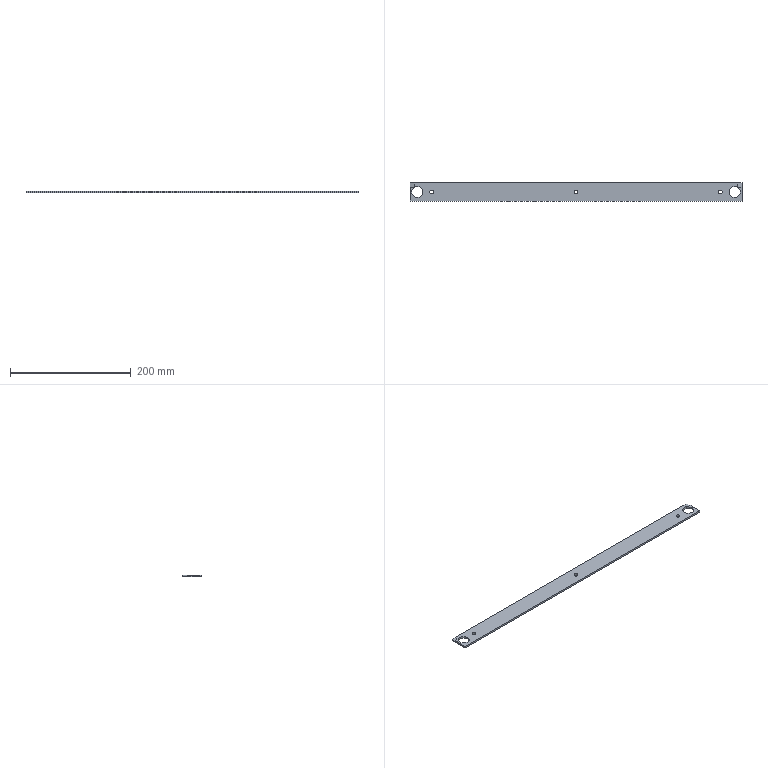Part | STEP file | 602-01-0036 | 1 solid | 20 faces | box 550 x 30 x 3 mm | volume 47601 mm3 | cylinder 10 | plane 10 | commonest cylinder face diameters 6.5 x6 18 x4